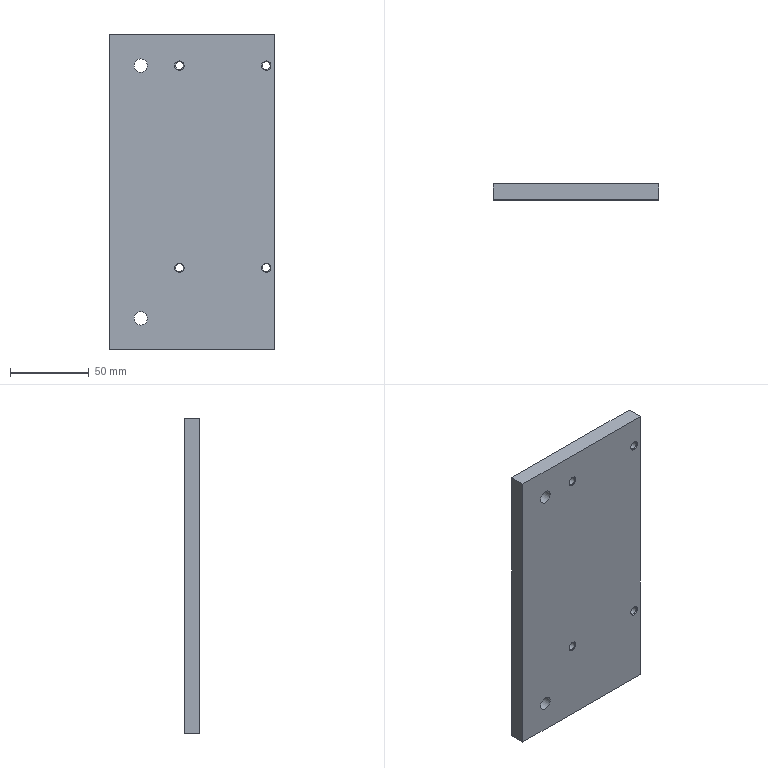Part | STEP file | Button box plate | 1 solid | 20 faces | box 105 x 10 x 200 mm | volume 208063 mm3 | cone 8 | cylinder 6 | plane 6 | commonest cylinder face diameters 5 x4 8.5 x2
STEP:
#1=CARTESIAN_POINT('',(0.,0.,0.));
#2=DIRECTION('',(0.,0.,1.));
#3=DIRECTION('',(1.,0.,0.));
#4=AXIS2_PLACEMENT_3D('',#1,#2,#3);
#5=CARTESIAN_POINT('',(-810.5,-295.,282.25));
#6=VERTEX_POINT('',#5);
#7=CARTESIAN_POINT('',(-810.5,-295.,278.));
#8=DIRECTION('',(0.,-1.,0.));
#9=DIRECTION('',(0.,0.,1.));
#10=AXIS2_PLACEMENT_3D('',#7,#8,#9);
#11=CIRCLE('',#10,4.25);
#12=CARTESIAN_POINT('',(-810.5,-328.,278.));
#13=DIRECTION('',(0.,1.,0.));
#14=DIRECTION('',(0.,0.,1.));
#15=AXIS2_PLACEMENT_3D('',#12,#13,#14);
#16=CYLINDRICAL_SURFACE('',#15,4.25);
#17=CARTESIAN_POINT('',(6.283,33.));
#18=DIRECTION('',(-1.,0.));
#19=VECTOR('',#18,1.);
#20=LINE('',#17,#19);
#21=(GEOMETRIC_REPRESENTATION_CONTEXT(2)PARAMETRIC_REPRESENTATION_CONTEXT()REPRESENTATION_CONTEXT('',''));
#22=DEFINITIONAL_REPRESENTATION('',(#20),#21);
#23=PCURVE('',#16,#22);
#24=CARTESIAN_POINT('',(-783.5,-295.,146.));
#25=DIRECTION('',(0.,1.,0.));
#26=DIRECTION('',(0.,0.,-1.));
#27=AXIS2_PLACEMENT_3D('',#24,#25,#26);
#28=PLANE('',#27);
#29=CARTESIAN_POINT('',(-136.25,27.));
#30=CARTESIAN_POINT('',(-136.25,34.361));
#31=CARTESIAN_POINT('',(-129.875,30.681));
#32=CARTESIAN_POINT('',(-123.5,27.));
#33=CARTESIAN_POINT('',(-129.875,23.319));
#34=CARTESIAN_POINT('',(-136.25,19.639));
#35=CARTESIAN_POINT('',(-136.25,27.));
#36=(BOUNDED_CURVE()B_SPLINE_CURVE(2,(#29,#30,#31,#32,#33,#34,#35),.UNSPECIFIED.,.T.,.F.)B_SPLINE_CURVE_WITH_KNOTS((1,2,2,2,2,1),(-2.094,0.,2.094,4.189,6.283,8.378),.UNSPECIFIED.)CURVE()GEOMETRIC_REPRESENTATION_ITEM()RATIONAL_B_SPLINE_CURVE((1.,0.5,1.,0.5,1.,0.5,1.))REPRESENTATION_ITEM(''));
#37=(GEOMETRIC_REPRESENTATION_CONTEXT(2)PARAMETRIC_REPRESENTATION_CONTEXT()REPRESENTATION_CONTEXT('',''));
#38=DEFINITIONAL_REPRESENTATION('',(#36),#37);
#39=PCURVE('',#28,#38);
#40=SURFACE_CURVE('',#11,(#23,#39),.PCURVE_S1.);
#41=EDGE_CURVE('',#6,#6,#40,.T.);
#42=ORIENTED_EDGE('',*,*,#41,.T.);
#43=CARTESIAN_POINT('',(-810.5,-305.,282.25));
#44=VERTEX_POINT('',#43);
#45=CARTESIAN_POINT('',(-810.5,-305.,282.25));
#46=CARTESIAN_POINT('',(-810.5,-295.,282.25));
#47=B_SPLINE_CURVE_WITH_KNOTS('',1,(#45,#46),.UNSPECIFIED.,.F.,.F.,(2,2),(23.,33.),.PIECEWISE_BEZIER_KNOTS.);
#48=CARTESIAN_POINT('',(0.,0.));
#49=DIRECTION('',(0.,1.));
#50=VECTOR('',#49,1.);
#51=LINE('',#48,#50);
#52=(GEOMETRIC_REPRESENTATION_CONTEXT(2)PARAMETRIC_REPRESENTATION_CONTEXT()REPRESENTATION_CONTEXT('',''));
#53=DEFINITIONAL_REPRESENTATION('',(#51),#52);
#54=PCURVE('',#16,#53);
#55=CARTESIAN_POINT('',(6.283,0.));
#56=DIRECTION('',(0.,1.));
#57=VECTOR('',#56,1.);
#58=LINE('',#55,#57);
#59=(GEOMETRIC_REPRESENTATION_CONTEXT(2)PARAMETRIC_REPRESENTATION_CONTEXT()REPRESENTATION_CONTEXT('',''));
#60=DEFINITIONAL_REPRESENTATION('',(#58),#59);
#61=PCURVE('',#16,#60);
#62=SEAM_CURVE('',#47,(#54,#61),.PCURVE_S1.);
#63=EDGE_CURVE('',#44,#6,#62,.T.);
#64=ORIENTED_EDGE('',*,*,#63,.F.);
#65=CARTESIAN_POINT('',(-810.5,-305.,278.));
#66=DIRECTION('',(0.,1.,0.));
#67=DIRECTION('',(0.,0.,1.));
#68=AXIS2_PLACEMENT_3D('',#65,#66,#67);
#69=CIRCLE('',#68,4.25);
#70=CARTESIAN_POINT('',(0.,23.));
#71=DIRECTION('',(1.,0.));
#72=VECTOR('',#71,1.);
#73=LINE('',#70,#72);
#74=(GEOMETRIC_REPRESENTATION_CONTEXT(2)PARAMETRIC_REPRESENTATION_CONTEXT()REPRESENTATION_CONTEXT('',''));
#75=DEFINITIONAL_REPRESENTATION('',(#73),#74);
#76=PCURVE('',#16,#75);
#77=CARTESIAN_POINT('',(-783.5,-305.,146.));
#78=DIRECTION('',(0.,1.,0.));
#79=DIRECTION('',(0.,0.,-1.));
#80=AXIS2_PLACEMENT_3D('',#77,#78,#79);
#81=PLANE('',#80);
#82=CARTESIAN_POINT('',(-132.,27.));
#83=DIRECTION('',(-1.,0.));
#84=AXIS2_PLACEMENT_2D('',#82,#83);
#85=CIRCLE('',#84,4.25);
#86=(GEOMETRIC_REPRESENTATION_CONTEXT(2)PARAMETRIC_REPRESENTATION_CONTEXT()REPRESENTATION_CONTEXT('',''));
#87=DEFINITIONAL_REPRESENTATION('',(#85),#86);
#88=PCURVE('',#81,#87);
#89=SURFACE_CURVE('',#69,(#76,#88),.PCURVE_S1.);
#90=EDGE_CURVE('',#44,#44,#89,.T.);
#91=ORIENTED_EDGE('',*,*,#90,.T.);
#92=ORIENTED_EDGE('',*,*,#63,.T.);
#93=EDGE_LOOP('',(#42,#64,#91,#92));
#94=FACE_BOUND('',#93,.F.);
#95=ADVANCED_FACE('',(#94),#16,.F.);
#96=CARTESIAN_POINT('',(-830.5,-305.,298.));
#97=VERTEX_POINT('',#96);
#98=CARTESIAN_POINT('',(-725.5,-305.,298.));
#99=VERTEX_POINT('',#98);
#100=CARTESIAN_POINT('',(-1441.,-305.,298.));
#101=DIRECTION('',(1.,0.,0.));
#102=VECTOR('',#101,1.);
#103=LINE('',#100,#102);
#104=CARTESIAN_POINT('',(-1441.,-107.5,298.));
#105=DIRECTION('',(0.,0.,-1.));
#106=DIRECTION('',(-1.,0.,0.));
#107=AXIS2_PLACEMENT_3D('',#104,#105,#106);
#108=PLANE('',#107);
#109=CARTESIAN_POINT('',(0.,-197.5));
#110=DIRECTION('',(-1.,0.));
#111=VECTOR('',#110,1.);
#112=LINE('',#109,#111);
#113=(GEOMETRIC_REPRESENTATION_CONTEXT(2)PARAMETRIC_REPRESENTATION_CONTEXT()REPRESENTATION_CONTEXT('',''));
#114=DEFINITIONAL_REPRESENTATION('',(#112),#113);
#115=PCURVE('',#108,#114);
#116=CARTESIAN_POINT('',(-152.,657.5));
#117=DIRECTION('',(0.,-1.));
#118=VECTOR('',#117,1.);
#119=LINE('',#116,#118);
#120=(GEOMETRIC_REPRESENTATION_CONTEXT(2)PARAMETRIC_REPRESENTATION_CONTEXT()REPRESENTATION_CONTEXT('',''));
#121=DEFINITIONAL_REPRESENTATION('',(#119),#120);
#122=PCURVE('',#81,#121);
#123=SURFACE_CURVE('',#103,(#115,#122),.PCURVE_S1.);
#124=EDGE_CURVE('',#97,#99,#123,.T.);
#125=ORIENTED_EDGE('',*,*,#124,.T.);
#126=CARTESIAN_POINT('',(-725.5,-295.,298.));
#127=VERTEX_POINT('',#126);
#128=CARTESIAN_POINT('',(-725.5,-107.5,298.));
#129=DIRECTION('',(0.,1.,0.));
#130=VECTOR('',#129,1.);
#131=LINE('',#128,#130);
#132=CARTESIAN_POINT('',(-715.5,0.));
#133=DIRECTION('',(0.,1.));
#134=VECTOR('',#133,1.);
#135=LINE('',#132,#134);
#136=(GEOMETRIC_REPRESENTATION_CONTEXT(2)PARAMETRIC_REPRESENTATION_CONTEXT()REPRESENTATION_CONTEXT('',''));
#137=DEFINITIONAL_REPRESENTATION('',(#135),#136);
#138=PCURVE('',#108,#137);
#139=CARTESIAN_POINT('',(-725.5,-295.,146.));
#140=DIRECTION('',(-1.,0.,0.));
#141=DIRECTION('',(0.,1.,0.));
#142=AXIS2_PLACEMENT_3D('',#139,#140,#141);
#143=PLANE('',#142);
#144=CARTESIAN_POINT('',(187.5,-152.));
#145=DIRECTION('',(1.,0.));
#146=VECTOR('',#145,1.);
#147=LINE('',#144,#146);
#148=(GEOMETRIC_REPRESENTATION_CONTEXT(2)PARAMETRIC_REPRESENTATION_CONTEXT()REPRESENTATION_CONTEXT('',''));
#149=DEFINITIONAL_REPRESENTATION('',(#147),#148);
#150=PCURVE('',#143,#149);
#151=SURFACE_CURVE('',#131,(#138,#150),.PCURVE_S1.);
#152=EDGE_CURVE('',#99,#127,#151,.T.);
#153=ORIENTED_EDGE('',*,*,#152,.T.);
#154=CARTESIAN_POINT('',(-830.5,-295.,298.));
#155=VERTEX_POINT('',#154);
#156=CARTESIAN_POINT('',(-1441.,-295.,298.));
#157=DIRECTION('',(1.,0.,0.));
#158=VECTOR('',#157,1.);
#159=LINE('',#156,#158);
#160=CARTESIAN_POINT('',(0.,-187.5));
#161=DIRECTION('',(-1.,0.));
#162=VECTOR('',#161,1.);
#163=LINE('',#160,#162);
#164=(GEOMETRIC_REPRESENTATION_CONTEXT(2)PARAMETRIC_REPRESENTATION_CONTEXT()REPRESENTATION_CONTEXT('',''));
#165=DEFINITIONAL_REPRESENTATION('',(#163),#164);
#166=PCURVE('',#108,#165);
#167=CARTESIAN_POINT('',(-152.,657.5));
#168=DIRECTION('',(0.,-1.));
#169=VECTOR('',#168,1.);
#170=LINE('',#167,#169);
#171=(GEOMETRIC_REPRESENTATION_CONTEXT(2)PARAMETRIC_REPRESENTATION_CONTEXT()REPRESENTATION_CONTEXT('',''));
#172=DEFINITIONAL_REPRESENTATION('',(#170),#171);
#173=PCURVE('',#28,#172);
#174=SURFACE_CURVE('',#159,(#166,#173),.PCURVE_S1.);
#175=EDGE_CURVE('',#155,#127,#174,.T.);
#176=ORIENTED_EDGE('',*,*,#175,.F.);
#177=CARTESIAN_POINT('',(-830.5,-295.,298.));
#178=DIRECTION('',(0.,1.,0.));
#179=VECTOR('',#178,1.);
#180=LINE('',#177,#179);
#181=CARTESIAN_POINT('',(-610.5,-187.5));
#182=DIRECTION('',(0.,1.));
#183=VECTOR('',#182,1.);
#184=LINE('',#181,#183);
#185=(GEOMETRIC_REPRESENTATION_CONTEXT(2)PARAMETRIC_REPRESENTATION_CONTEXT()REPRESENTATION_CONTEXT('',''));
#186=DEFINITIONAL_REPRESENTATION('',(#184),#185);
#187=PCURVE('',#108,#186);
#188=CARTESIAN_POINT('',(-830.5,-295.,294.));
#189=DIRECTION('',(1.,0.,0.));
#190=DIRECTION('',(0.,-1.,0.));
#191=AXIS2_PLACEMENT_3D('',#188,#189,#190);
#192=PLANE('',#191);
#193=CARTESIAN_POINT('',(0.,-4.));
#194=DIRECTION('',(-1.,0.));
#195=VECTOR('',#194,1.);
#196=LINE('',#193,#195);
#197=(GEOMETRIC_REPRESENTATION_CONTEXT(2)PARAMETRIC_REPRESENTATION_CONTEXT()REPRESENTATION_CONTEXT('',''));
#198=DEFINITIONAL_REPRESENTATION('',(#196),#197);
#199=PCURVE('',#192,#198);
#200=SURFACE_CURVE('',#180,(#187,#199),.PCURVE_S1.);
#201=EDGE_CURVE('',#97,#155,#200,.T.);
#202=ORIENTED_EDGE('',*,*,#201,.F.);
#203=EDGE_LOOP('',(#125,#153,#176,#202));
#204=FACE_BOUND('',#203,.T.);
#205=ADVANCED_FACE('',(#204),#108,.F.);
#206=CARTESIAN_POINT('',(-725.5,-305.,98.));
#207=VERTEX_POINT('',#206);
#208=CARTESIAN_POINT('',(-725.5,-305.,146.));
#209=DIRECTION('',(0.,0.,-1.));
#210=VECTOR('',#209,1.);
#211=LINE('',#208,#210);
#212=CARTESIAN_POINT('',(-10.,0.));
#213=DIRECTION('',(0.,1.));
#214=VECTOR('',#213,1.);
#215=LINE('',#212,#214);
#216=(GEOMETRIC_REPRESENTATION_CONTEXT(2)PARAMETRIC_REPRESENTATION_CONTEXT()REPRESENTATION_CONTEXT('',''));
#217=DEFINITIONAL_REPRESENTATION('',(#215),#216);
#218=PCURVE('',#143,#217);
#219=CARTESIAN_POINT('',(0.,-58.));
#220=DIRECTION('',(1.,0.));
#221=VECTOR('',#220,1.);
#222=LINE('',#219,#221);
#223=(GEOMETRIC_REPRESENTATION_CONTEXT(2)PARAMETRIC_REPRESENTATION_CONTEXT()REPRESENTATION_CONTEXT('',''));
#224=DEFINITIONAL_REPRESENTATION('',(#222),#223);
#225=PCURVE('',#81,#224);
#226=SURFACE_CURVE('',#211,(#218,#225),.PCURVE_S1.);
#227=EDGE_CURVE('',#99,#207,#226,.T.);
#228=ORIENTED_EDGE('',*,*,#227,.T.);
#229=CARTESIAN_POINT('',(-725.5,-295.,98.));
#230=VERTEX_POINT('',#229);
#231=CARTESIAN_POINT('',(-725.5,-295.,98.));
#232=DIRECTION('',(0.,1.,0.));
#233=VECTOR('',#232,1.);
#234=LINE('',#231,#233);
#235=CARTESIAN_POINT('',(0.,48.));
#236=DIRECTION('',(1.,0.));
#237=VECTOR('',#236,1.);
#238=LINE('',#235,#237);
#239=(GEOMETRIC_REPRESENTATION_CONTEXT(2)PARAMETRIC_REPRESENTATION_CONTEXT()REPRESENTATION_CONTEXT('',''));
#240=DEFINITIONAL_REPRESENTATION('',(#238),#239);
#241=PCURVE('',#143,#240);
#242=CARTESIAN_POINT('',(-798.5,-375.,98.));
#243=DIRECTION('',(0.,0.,1.));
#244=DIRECTION('',(0.,1.,0.));
#245=AXIS2_PLACEMENT_3D('',#242,#243,#244);
#246=PLANE('',#245);
#247=CARTESIAN_POINT('',(80.,-73.));
#248=DIRECTION('',(1.,0.));
#249=VECTOR('',#248,1.);
#250=LINE('',#247,#249);
#251=(GEOMETRIC_REPRESENTATION_CONTEXT(2)PARAMETRIC_REPRESENTATION_CONTEXT()REPRESENTATION_CONTEXT('',''));
#252=DEFINITIONAL_REPRESENTATION('',(#250),#251);
#253=PCURVE('',#246,#252);
#254=SURFACE_CURVE('',#234,(#241,#253),.PCURVE_S1.);
#255=EDGE_CURVE('',#207,#230,#254,.T.);
#256=ORIENTED_EDGE('',*,*,#255,.T.);
#257=CARTESIAN_POINT('',(-725.5,-295.,146.));
#258=DIRECTION('',(0.,0.,-1.));
#259=VECTOR('',#258,1.);
#260=LINE('',#257,#259);
#261=CARTESIAN_POINT('',(0.,0.));
#262=DIRECTION('',(0.,1.));
#263=VECTOR('',#262,1.);
#264=LINE('',#261,#263);
#265=(GEOMETRIC_REPRESENTATION_CONTEXT(2)PARAMETRIC_REPRESENTATION_CONTEXT()REPRESENTATION_CONTEXT('',''));
#266=DEFINITIONAL_REPRESENTATION('',(#264),#265);
#267=PCURVE('',#143,#266);
#268=CARTESIAN_POINT('',(0.,-58.));
#269=DIRECTION('',(1.,0.));
#270=VECTOR('',#269,1.);
#271=LINE('',#268,#270);
#272=(GEOMETRIC_REPRESENTATION_CONTEXT(2)PARAMETRIC_REPRESENTATION_CONTEXT()REPRESENTATION_CONTEXT('',''));
#273=DEFINITIONAL_REPRESENTATION('',(#271),#272);
#274=PCURVE('',#28,#273);
#275=SURFACE_CURVE('',#260,(#267,#274),.PCURVE_S1.);
#276=EDGE_CURVE('',#127,#230,#275,.T.);
#277=ORIENTED_EDGE('',*,*,#276,.F.);
#278=ORIENTED_EDGE('',*,*,#152,.F.);
#279=EDGE_LOOP('',(#228,#256,#277,#278));
#280=FACE_BOUND('',#279,.T.);
#281=ADVANCED_FACE('',(#280),#143,.F.);
#282=CARTESIAN_POINT('',(-830.5,-305.,98.));
#283=VERTEX_POINT('',#282);
#284=CARTESIAN_POINT('',(-798.5,-305.,98.));
#285=DIRECTION('',(-1.,0.,0.));
#286=VECTOR('',#285,1.);
#287=LINE('',#284,#286);
#288=CARTESIAN_POINT('',(70.,0.));
#289=DIRECTION('',(0.,1.));
#290=VECTOR('',#289,1.);
#291=LINE('',#288,#290);
#292=(GEOMETRIC_REPRESENTATION_CONTEXT(2)PARAMETRIC_REPRESENTATION_CONTEXT()REPRESENTATION_CONTEXT('',''));
#293=DEFINITIONAL_REPRESENTATION('',(#291),#292);
#294=PCURVE('',#246,#293);
#295=CARTESIAN_POINT('',(48.,15.));
#296=DIRECTION('',(0.,1.));
#297=VECTOR('',#296,1.);
#298=LINE('',#295,#297);
#299=(GEOMETRIC_REPRESENTATION_CONTEXT(2)PARAMETRIC_REPRESENTATION_CONTEXT()REPRESENTATION_CONTEXT('',''));
#300=DEFINITIONAL_REPRESENTATION('',(#298),#299);
#301=PCURVE('',#81,#300);
#302=SURFACE_CURVE('',#287,(#294,#301),.PCURVE_S1.);
#303=EDGE_CURVE('',#207,#283,#302,.T.);
#304=ORIENTED_EDGE('',*,*,#303,.T.);
#305=CARTESIAN_POINT('',(-830.5,-295.,98.));
#306=VERTEX_POINT('',#305);
#307=CARTESIAN_POINT('',(-830.5,-375.,98.));
#308=DIRECTION('',(0.,1.,0.));
#309=VECTOR('',#308,1.);
#310=LINE('',#307,#309);
#311=CARTESIAN_POINT('',(0.,32.));
#312=DIRECTION('',(1.,0.));
#313=VECTOR('',#312,1.);
#314=LINE('',#311,#313);
#315=(GEOMETRIC_REPRESENTATION_CONTEXT(2)PARAMETRIC_REPRESENTATION_CONTEXT()REPRESENTATION_CONTEXT('',''));
#316=DEFINITIONAL_REPRESENTATION('',(#314),#315);
#317=PCURVE('',#246,#316);
#318=CARTESIAN_POINT('',(80.,196.));
#319=DIRECTION('',(-1.,0.));
#320=VECTOR('',#319,1.);
#321=LINE('',#318,#320);
#322=(GEOMETRIC_REPRESENTATION_CONTEXT(2)PARAMETRIC_REPRESENTATION_CONTEXT()REPRESENTATION_CONTEXT('',''));
#323=DEFINITIONAL_REPRESENTATION('',(#321),#322);
#324=PCURVE('',#192,#323);
#325=SURFACE_CURVE('',#310,(#317,#324),.PCURVE_S1.);
#326=EDGE_CURVE('',#283,#306,#325,.T.);
#327=ORIENTED_EDGE('',*,*,#326,.T.);
#328=CARTESIAN_POINT('',(-798.5,-295.,98.));
#329=DIRECTION('',(-1.,0.,0.));
#330=VECTOR('',#329,1.);
#331=LINE('',#328,#330);
#332=CARTESIAN_POINT('',(80.,0.));
#333=DIRECTION('',(0.,1.));
#334=VECTOR('',#333,1.);
#335=LINE('',#332,#334);
#336=(GEOMETRIC_REPRESENTATION_CONTEXT(2)PARAMETRIC_REPRESENTATION_CONTEXT()REPRESENTATION_CONTEXT('',''));
#337=DEFINITIONAL_REPRESENTATION('',(#335),#336);
#338=PCURVE('',#246,#337);
#339=CARTESIAN_POINT('',(48.,15.));
#340=DIRECTION('',(0.,1.));
#341=VECTOR('',#340,1.);
#342=LINE('',#339,#341);
#343=(GEOMETRIC_REPRESENTATION_CONTEXT(2)PARAMETRIC_REPRESENTATION_CONTEXT()REPRESENTATION_CONTEXT('',''));
#344=DEFINITIONAL_REPRESENTATION('',(#342),#343);
#345=PCURVE('',#28,#344);
#346=SURFACE_CURVE('',#331,(#338,#345),.PCURVE_S1.);
#347=EDGE_CURVE('',#230,#306,#346,.T.);
#348=ORIENTED_EDGE('',*,*,#347,.F.);
#349=ORIENTED_EDGE('',*,*,#255,.F.);
#350=EDGE_LOOP('',(#304,#327,#348,#349));
#351=FACE_BOUND('',#350,.T.);
#352=ADVANCED_FACE('',(#351),#246,.F.);
#353=CARTESIAN_POINT('',(-830.5,-305.,294.));
#354=DIRECTION('',(0.,0.,1.));
#355=VECTOR('',#354,1.);
#356=LINE('',#353,#355);
#357=CARTESIAN_POINT('',(10.,0.));
#358=DIRECTION('',(0.,-1.));
#359=VECTOR('',#358,1.);
#360=LINE('',#357,#359);
#361=(GEOMETRIC_REPRESENTATION_CONTEXT(2)PARAMETRIC_REPRESENTATION_CONTEXT()REPRESENTATION_CONTEXT('',''));
#362=DEFINITIONAL_REPRESENTATION('',(#360),#361);
#363=PCURVE('',#192,#362);
#364=CARTESIAN_POINT('',(-148.,47.));
#365=DIRECTION('',(-1.,0.));
#366=VECTOR('',#365,1.);
#367=LINE('',#364,#366);
#368=(GEOMETRIC_REPRESENTATION_CONTEXT(2)PARAMETRIC_REPRESENTATION_CONTEXT()REPRESENTATION_CONTEXT('',''));
#369=DEFINITIONAL_REPRESENTATION('',(#367),#368);
#370=PCURVE('',#81,#369);
#371=SURFACE_CURVE('',#356,(#363,#370),.PCURVE_S1.);
#372=EDGE_CURVE('',#283,#97,#371,.T.);
#373=ORIENTED_EDGE('',*,*,#372,.T.);
#374=ORIENTED_EDGE('',*,*,#201,.T.);
#375=CARTESIAN_POINT('',(-830.5,-295.,294.));
#376=DIRECTION('',(0.,0.,1.));
#377=VECTOR('',#376,1.);
#378=LINE('',#375,#377);
#379=CARTESIAN_POINT('',(0.,0.));
#380=DIRECTION('',(0.,-1.));
#381=VECTOR('',#380,1.);
#382=LINE('',#379,#381);
#383=(GEOMETRIC_REPRESENTATION_CONTEXT(2)PARAMETRIC_REPRESENTATION_CONTEXT()REPRESENTATION_CONTEXT('',''));
#384=DEFINITIONAL_REPRESENTATION('',(#382),#383);
#385=PCURVE('',#192,#384);
#386=CARTESIAN_POINT('',(-148.,47.));
#387=DIRECTION('',(-1.,0.));
#388=VECTOR('',#387,1.);
#389=LINE('',#386,#388);
#390=(GEOMETRIC_REPRESENTATION_CONTEXT(2)PARAMETRIC_REPRESENTATION_CONTEXT()REPRESENTATION_CONTEXT('',''));
#391=DEFINITIONAL_REPRESENTATION('',(#389),#390);
#392=PCURVE('',#28,#391);
#393=SURFACE_CURVE('',#378,(#385,#392),.PCURVE_S1.);
#394=EDGE_CURVE('',#306,#155,#393,.T.);
#395=ORIENTED_EDGE('',*,*,#394,.F.);
#396=ORIENTED_EDGE('',*,*,#326,.F.);
#397=EDGE_LOOP('',(#373,#374,#395,#396));
#398=FACE_BOUND('',#397,.T.);
#399=ADVANCED_FACE('',(#398),#192,.F.);
#400=CARTESIAN_POINT('',(-786.,-305.,281.));
#401=VERTEX_POINT('',#400);
#402=CARTESIAN_POINT('',(-786.,-305.,278.));
#403=DIRECTION('',(0.,1.,0.));
#404=DIRECTION('',(0.,0.,1.));
#405=AXIS2_PLACEMENT_3D('',#402,#403,#404);
#406=CIRCLE('',#405,3.);
#407=CARTESIAN_POINT('',(-132.,2.5));
#408=DIRECTION('',(-1.,0.));
#409=AXIS2_PLACEMENT_2D('',#407,#408);
#410=CIRCLE('',#409,3.);
#411=(GEOMETRIC_REPRESENTATION_CONTEXT(2)PARAMETRIC_REPRESENTATION_CONTEXT()REPRESENTATION_CONTEXT('',''));
#412=DEFINITIONAL_REPRESENTATION('',(#410),#411);
#413=PCURVE('',#81,#412);
#414=CARTESIAN_POINT('',(-786.,-304.5,278.));
#415=DIRECTION('',(0.,-1.,0.));
#416=DIRECTION('',(0.,0.,-1.));
#417=AXIS2_PLACEMENT_3D('',#414,#415,#416);
#418=CONICAL_SURFACE('',#417,2.5,0.7854);
#419=CARTESIAN_POINT('',(9.425,0.5));
#420=DIRECTION('',(-1.,0.));
#421=VECTOR('',#420,1.);
#422=LINE('',#419,#421);
#423=(GEOMETRIC_REPRESENTATION_CONTEXT(2)PARAMETRIC_REPRESENTATION_CONTEXT()REPRESENTATION_CONTEXT('',''));
#424=DEFINITIONAL_REPRESENTATION('',(#422),#423);
#425=PCURVE('',#418,#424);
#426=SURFACE_CURVE('',#406,(#413,#425),.PCURVE_S1.);
#427=EDGE_CURVE('',#401,#401,#426,.T.);
#428=ORIENTED_EDGE('',*,*,#427,.T.);
#429=EDGE_LOOP('',(#428));
#430=FACE_BOUND('',#429,.T.);
#431=CARTESIAN_POINT('',(-731.,-305.,281.));
#432=VERTEX_POINT('',#431);
#433=CARTESIAN_POINT('',(-731.,-305.,278.));
#434=DIRECTION('',(0.,1.,0.));
#435=DIRECTION('',(0.,0.,1.));
#436=AXIS2_PLACEMENT_3D('',#433,#434,#435);
#437=CIRCLE('',#436,3.);
#438=CARTESIAN_POINT('',(-132.,-52.5));
#439=DIRECTION('',(-1.,0.));
#440=AXIS2_PLACEMENT_2D('',#438,#439);
#441=CIRCLE('',#440,3.);
#442=(GEOMETRIC_REPRESENTATION_CONTEXT(2)PARAMETRIC_REPRESENTATION_CONTEXT()REPRESENTATION_CONTEXT('',''));
#443=DEFINITIONAL_REPRESENTATION('',(#441),#442);
#444=PCURVE('',#81,#443);
#445=CARTESIAN_POINT('',(-731.,-304.5,278.));
#446=DIRECTION('',(0.,-1.,0.));
#447=DIRECTION('',(0.,0.,-1.));
#448=AXIS2_PLACEMENT_3D('',#445,#446,#447);
#449=CONICAL_SURFACE('',#448,2.5,0.7854);
#450=CARTESIAN_POINT('',(9.425,0.5));
#451=DIRECTION('',(-1.,0.));
#452=VECTOR('',#451,1.);
#453=LINE('',#450,#452);
#454=(GEOMETRIC_REPRESENTATION_CONTEXT(2)PARAMETRIC_REPRESENTATION_CONTEXT()REPRESENTATION_CONTEXT('',''));
#455=DEFINITIONAL_REPRESENTATION('',(#453),#454);
#456=PCURVE('',#449,#455);
#457=SURFACE_CURVE('',#437,(#444,#456),.PCURVE_S1.);
#458=EDGE_CURVE('',#432,#432,#457,.T.);
#459=ORIENTED_EDGE('',*,*,#458,.T.);
#460=EDGE_LOOP('',(#459));
#461=FACE_BOUND('',#460,.T.);
#462=CARTESIAN_POINT('',(-731.,-305.,153.));
#463=VERTEX_POINT('',#462);
#464=CARTESIAN_POINT('',(-731.,-305.,150.));
#465=DIRECTION('',(0.,1.,0.));
#466=DIRECTION('',(0.,0.,1.));
#467=AXIS2_PLACEMENT_3D('',#464,#465,#466);
#468=CIRCLE('',#467,3.);
#469=CARTESIAN_POINT('',(-4.,-52.5));
#470=DIRECTION('',(-1.,0.));
#471=AXIS2_PLACEMENT_2D('',#469,#470);
#472=CIRCLE('',#471,3.);
#473=(GEOMETRIC_REPRESENTATION_CONTEXT(2)PARAMETRIC_REPRESENTATION_CONTEXT()REPRESENTATION_CONTEXT('',''));
#474=DEFINITIONAL_REPRESENTATION('',(#472),#473);
#475=PCURVE('',#81,#474);
#476=CARTESIAN_POINT('',(-731.,-304.5,150.));
#477=DIRECTION('',(0.,-1.,0.));
#478=DIRECTION('',(0.,0.,-1.));
#479=AXIS2_PLACEMENT_3D('',#476,#477,#478);
#480=CONICAL_SURFACE('',#479,2.5,0.7854);
#481=CARTESIAN_POINT('',(9.425,0.5));
#482=DIRECTION('',(-1.,0.));
#483=VECTOR('',#482,1.);
#484=LINE('',#481,#483);
#485=(GEOMETRIC_REPRESENTATION_CONTEXT(2)PARAMETRIC_REPRESENTATION_CONTEXT()REPRESENTATION_CONTEXT('',''));
#486=DEFINITIONAL_REPRESENTATION('',(#484),#485);
#487=PCURVE('',#480,#486);
#488=SURFACE_CURVE('',#468,(#475,#487),.PCURVE_S1.);
#489=EDGE_CURVE('',#463,#463,#488,.T.);
#490=ORIENTED_EDGE('',*,*,#489,.T.);
#491=EDGE_LOOP('',(#490));
#492=FACE_BOUND('',#491,.T.);
#493=CARTESIAN_POINT('',(-786.,-305.,153.));
#494=VERTEX_POINT('',#493);
#495=CARTESIAN_POINT('',(-786.,-305.,150.));
#496=DIRECTION('',(0.,1.,0.));
#497=DIRECTION('',(0.,0.,1.));
#498=AXIS2_PLACEMENT_3D('',#495,#496,#497);
#499=CIRCLE('',#498,3.);
#500=CARTESIAN_POINT('',(-4.,2.5));
#501=DIRECTION('',(-1.,0.));
#502=AXIS2_PLACEMENT_2D('',#500,#501);
#503=CIRCLE('',#502,3.);
#504=(GEOMETRIC_REPRESENTATION_CONTEXT(2)PARAMETRIC_REPRESENTATION_CONTEXT()REPRESENTATION_CONTEXT('',''));
#505=DEFINITIONAL_REPRESENTATION('',(#503),#504);
#506=PCURVE('',#81,#505);
#507=CARTESIAN_POINT('',(-786.,-304.5,150.));
#508=DIRECTION('',(0.,-1.,0.));
#509=DIRECTION('',(0.,0.,-1.));
#510=AXIS2_PLACEMENT_3D('',#507,#508,#509);
#511=CONICAL_SURFACE('',#510,2.5,0.7854);
#512=CARTESIAN_POINT('',(9.425,0.5));
#513=DIRECTION('',(-1.,0.));
#514=VECTOR('',#513,1.);
#515=LINE('',#512,#514);
#516=(GEOMETRIC_REPRESENTATION_CONTEXT(2)PARAMETRIC_REPRESENTATION_CONTEXT()REPRESENTATION_CONTEXT('',''));
#517=DEFINITIONAL_REPRESENTATION('',(#515),#516);
#518=PCURVE('',#511,#517);
#519=SURFACE_CURVE('',#499,(#506,#518),.PCURVE_S1.);
#520=EDGE_CURVE('',#494,#494,#519,.T.);
#521=ORIENTED_EDGE('',*,*,#520,.T.);
#522=EDGE_LOOP('',(#521));
#523=FACE_BOUND('',#522,.T.);
#524=CARTESIAN_POINT('',(-810.5,-305.,122.25));
#525=VERTEX_POINT('',#524);
#526=CARTESIAN_POINT('',(-810.5,-305.,118.));
#527=DIRECTION('',(0.,1.,0.));
#528=DIRECTION('',(0.,0.,1.));
#529=AXIS2_PLACEMENT_3D('',#526,#527,#528);
#530=CIRCLE('',#529,4.25);
#531=CARTESIAN_POINT('',(28.,27.));
#532=DIRECTION('',(-1.,0.));
#533=AXIS2_PLACEMENT_2D('',#531,#532);
#534=CIRCLE('',#533,4.25);
#535=(GEOMETRIC_REPRESENTATION_CONTEXT(2)PARAMETRIC_REPRESENTATION_CONTEXT()REPRESENTATION_CONTEXT('',''));
#536=DEFINITIONAL_REPRESENTATION('',(#534),#535);
#537=PCURVE('',#81,#536);
#538=CARTESIAN_POINT('',(-810.5,-328.,118.));
#539=DIRECTION('',(0.,1.,0.));
#540=DIRECTION('',(0.,0.,1.));
#541=AXIS2_PLACEMENT_3D('',#538,#539,#540);
#542=CYLINDRICAL_SURFACE('',#541,4.25);
#543=CARTESIAN_POINT('',(0.,23.));
#544=DIRECTION('',(1.,0.));
#545=VECTOR('',#544,1.);
#546=LINE('',#543,#545);
#547=(GEOMETRIC_REPRESENTATION_CONTEXT(2)PARAMETRIC_REPRESENTATION_CONTEXT()REPRESENTATION_CONTEXT('',''));
#548=DEFINITIONAL_REPRESENTATION('',(#546),#547);
#549=PCURVE('',#542,#548);
#550=SURFACE_CURVE('',#530,(#537,#549),.PCURVE_S1.);
#551=EDGE_CURVE('',#525,#525,#550,.T.);
#552=ORIENTED_EDGE('',*,*,#551,.T.);
#553=EDGE_LOOP('',(#552));
#554=FACE_BOUND('',#553,.T.);
#555=ORIENTED_EDGE('',*,*,#90,.T.);
#556=EDGE_LOOP('',(#555));
#557=FACE_BOUND('',#556,.T.);
#558=ORIENTED_EDGE('',*,*,#372,.F.);
#559=ORIENTED_EDGE('',*,*,#303,.F.);
#560=ORIENTED_EDGE('',*,*,#227,.F.);
#561=ORIENTED_EDGE('',*,*,#124,.F.);
#562=EDGE_LOOP('',(#558,#559,#560,#561));
#563=FACE_BOUND('',#562,.T.);
#564=ADVANCED_FACE('',(#430,#461,#492,#523,#554,#557,#563),#81,.F.);
#565=CARTESIAN_POINT('',(-786.,-295.,281.));
#566=VERTEX_POINT('',#565);
#567=CARTESIAN_POINT('',(-786.,-295.,278.));
#568=DIRECTION('',(0.,-1.,0.));
#569=DIRECTION('',(0.,0.,1.));
#570=AXIS2_PLACEMENT_3D('',#567,#568,#569);
#571=CIRCLE('',#570,3.);
#572=CARTESIAN_POINT('',(-135.,2.5));
#573=CARTESIAN_POINT('',(-135.,7.696));
#574=CARTESIAN_POINT('',(-130.5,5.098));
#575=CARTESIAN_POINT('',(-126.,2.5));
#576=CARTESIAN_POINT('',(-130.5,-0.09808));
#577=CARTESIAN_POINT('',(-135.,-2.696));
#578=CARTESIAN_POINT('',(-135.,2.5));
#579=(BOUNDED_CURVE()B_SPLINE_CURVE(2,(#572,#573,#574,#575,#576,#577,#578),.UNSPECIFIED.,.T.,.F.)B_SPLINE_CURVE_WITH_KNOTS((1,2,2,2,2,1),(-2.094,0.,2.094,4.189,6.283,8.378),.UNSPECIFIED.)CURVE()GEOMETRIC_REPRESENTATION_ITEM()RATIONAL_B_SPLINE_CURVE((1.,0.5,1.,0.5,1.,0.5,1.))REPRESENTATION_ITEM(''));
#580=(GEOMETRIC_REPRESENTATION_CONTEXT(2)PARAMETRIC_REPRESENTATION_CONTEXT()REPRESENTATION_CONTEXT('',''));
#581=DEFINITIONAL_REPRESENTATION('',(#579),#580);
#582=PCURVE('',#28,#581);
#583=CARTESIAN_POINT('',(-786.,-295.,278.));
#584=DIRECTION('',(0.,1.,0.));
#585=DIRECTION('',(0.,0.,1.));
#586=AXIS2_PLACEMENT_3D('',#583,#584,#585);
#587=CONICAL_SURFACE('',#586,3.,0.7854);
#588=CARTESIAN_POINT('',(6.283,0.));
#589=DIRECTION('',(-1.,0.));
#590=VECTOR('',#589,1.);
#591=LINE('',#588,#590);
#592=(GEOMETRIC_REPRESENTATION_CONTEXT(2)PARAMETRIC_REPRESENTATION_CONTEXT()REPRESENTATION_CONTEXT('',''));
#593=DEFINITIONAL_REPRESENTATION('',(#591),#592);
#594=PCURVE('',#587,#593);
#595=SURFACE_CURVE('',#571,(#582,#594),.PCURVE_S1.);
#596=EDGE_CURVE('',#566,#566,#595,.T.);
#597=ORIENTED_EDGE('',*,*,#596,.T.);
#598=EDGE_LOOP('',(#597));
#599=FACE_BOUND('',#598,.T.);
#600=CARTESIAN_POINT('',(-731.,-295.,281.));
#601=VERTEX_POINT('',#600);
#602=CARTESIAN_POINT('',(-731.,-295.,278.));
#603=DIRECTION('',(0.,-1.,0.));
#604=DIRECTION('',(0.,0.,1.));
#605=AXIS2_PLACEMENT_3D('',#602,#603,#604);
#606=CIRCLE('',#605,3.);
#607=CARTESIAN_POINT('',(-135.,-52.5));
#608=CARTESIAN_POINT('',(-135.,-47.304));
#609=CARTESIAN_POINT('',(-130.5,-49.902));
#610=CARTESIAN_POINT('',(-126.,-52.5));
#611=CARTESIAN_POINT('',(-130.5,-55.098));
#612=CARTESIAN_POINT('',(-135.,-57.696));
#613=CARTESIAN_POINT('',(-135.,-52.5));
#614=(BOUNDED_CURVE()B_SPLINE_CURVE(2,(#607,#608,#609,#610,#611,#612,#613),.UNSPECIFIED.,.T.,.F.)B_SPLINE_CURVE_WITH_KNOTS((1,2,2,2,2,1),(-2.094,0.,2.094,4.189,6.283,8.378),.UNSPECIFIED.)CURVE()GEOMETRIC_REPRESENTATION_ITEM()RATIONAL_B_SPLINE_CURVE((1.,0.5,1.,0.5,1.,0.5,1.))REPRESENTATION_ITEM(''));
#615=(GEOMETRIC_REPRESENTATION_CONTEXT(2)PARAMETRIC_REPRESENTATION_CONTEXT()REPRESENTATION_CONTEXT('',''));
#616=DEFINITIONAL_REPRESENTATION('',(#614),#615);
#617=PCURVE('',#28,#616);
#618=CARTESIAN_POINT('',(-731.,-295.,278.));
#619=DIRECTION('',(0.,1.,0.));
#620=DIRECTION('',(0.,0.,1.));
#621=AXIS2_PLACEMENT_3D('',#618,#619,#620);
#622=CONICAL_SURFACE('',#621,3.,0.7854);
#623=CARTESIAN_POINT('',(6.283,0.));
#624=DIRECTION('',(-1.,0.));
#625=VECTOR('',#624,1.);
#626=LINE('',#623,#625);
#627=(GEOMETRIC_REPRESENTATION_CONTEXT(2)PARAMETRIC_REPRESENTATION_CONTEXT()REPRESENTATION_CONTEXT('',''));
#628=DEFINITIONAL_REPRESENTATION('',(#626),#627);
#629=PCURVE('',#622,#628);
#630=SURFACE_CURVE('',#606,(#617,#629),.PCURVE_S1.);
#631=EDGE_CURVE('',#601,#601,#630,.T.);
#632=ORIENTED_EDGE('',*,*,#631,.T.);
#633=EDGE_LOOP('',(#632));
#634=FACE_BOUND('',#633,.T.);
#635=CARTESIAN_POINT('',(-731.,-295.,153.));
#636=VERTEX_POINT('',#635);
#637=CARTESIAN_POINT('',(-731.,-295.,150.));
#638=DIRECTION('',(0.,-1.,0.));
#639=DIRECTION('',(0.,0.,1.));
#640=AXIS2_PLACEMENT_3D('',#637,#638,#639);
#641=CIRCLE('',#640,3.);
#642=CARTESIAN_POINT('',(-7.,-52.5));
#643=CARTESIAN_POINT('',(-7.,-47.304));
#644=CARTESIAN_POINT('',(-2.5,-49.902));
#645=CARTESIAN_POINT('',(2.,-52.5));
#646=CARTESIAN_POINT('',(-2.5,-55.098));
#647=CARTESIAN_POINT('',(-7.,-57.696));
#648=CARTESIAN_POINT('',(-7.,-52.5));
#649=(BOUNDED_CURVE()B_SPLINE_CURVE(2,(#642,#643,#644,#645,#646,#647,#648),.UNSPECIFIED.,.T.,.F.)B_SPLINE_CURVE_WITH_KNOTS((1,2,2,2,2,1),(-2.094,0.,2.094,4.189,6.283,8.378),.UNSPECIFIED.)CURVE()GEOMETRIC_REPRESENTATION_ITEM()RATIONAL_B_SPLINE_CURVE((1.,0.5,1.,0.5,1.,0.5,1.))REPRESENTATION_ITEM(''));
#650=(GEOMETRIC_REPRESENTATION_CONTEXT(2)PARAMETRIC_REPRESENTATION_CONTEXT()REPRESENTATION_CONTEXT('',''));
#651=DEFINITIONAL_REPRESENTATION('',(#649),#650);
#652=PCURVE('',#28,#651);
#653=CARTESIAN_POINT('',(-731.,-295.,150.));
#654=DIRECTION('',(0.,1.,0.));
#655=DIRECTION('',(0.,0.,1.));
#656=AXIS2_PLACEMENT_3D('',#653,#654,#655);
#657=CONICAL_SURFACE('',#656,3.,0.7854);
#658=CARTESIAN_POINT('',(6.283,0.));
#659=DIRECTION('',(-1.,0.));
#660=VECTOR('',#659,1.);
#661=LINE('',#658,#660);
#662=(GEOMETRIC_REPRESENTATION_CONTEXT(2)PARAMETRIC_REPRESENTATION_CONTEXT()REPRESENTATION_CONTEXT('',''));
#663=DEFINITIONAL_REPRESENTATION('',(#661),#662);
#664=PCURVE('',#657,#663);
#665=SURFACE_CURVE('',#641,(#652,#664),.PCURVE_S1.);
#666=EDGE_CURVE('',#636,#636,#665,.T.);
#667=ORIENTED_EDGE('',*,*,#666,.T.);
#668=EDGE_LOOP('',(#667));
#669=FACE_BOUND('',#668,.T.);
#670=CARTESIAN_POINT('',(-786.,-295.,153.));
#671=VERTEX_POINT('',#670);
#672=CARTESIAN_POINT('',(-786.,-295.,150.));
#673=DIRECTION('',(0.,-1.,0.));
#674=DIRECTION('',(0.,0.,1.));
#675=AXIS2_PLACEMENT_3D('',#672,#673,#674);
#676=CIRCLE('',#675,3.);
#677=CARTESIAN_POINT('',(-7.,2.5));
#678=CARTESIAN_POINT('',(-7.,7.696));
#679=CARTESIAN_POINT('',(-2.5,5.098));
#680=CARTESIAN_POINT('',(2.,2.5));
#681=CARTESIAN_POINT('',(-2.5,-0.09808));
#682=CARTESIAN_POINT('',(-7.,-2.696));
#683=CARTESIAN_POINT('',(-7.,2.5));
#684=(BOUNDED_CURVE()B_SPLINE_CURVE(2,(#677,#678,#679,#680,#681,#682,#683),.UNSPECIFIED.,.T.,.F.)B_SPLINE_CURVE_WITH_KNOTS((1,2,2,2,2,1),(-2.094,0.,2.094,4.189,6.283,8.378),.UNSPECIFIED.)CURVE()GEOMETRIC_REPRESENTATION_ITEM()RATIONAL_B_SPLINE_CURVE((1.,0.5,1.,0.5,1.,0.5,1.))REPRESENTATION_ITEM(''));
#685=(GEOMETRIC_REPRESENTATION_CONTEXT(2)PARAMETRIC_REPRESENTATION_CONTEXT()REPRESENTATION_CONTEXT('',''));
#686=DEFINITIONAL_REPRESENTATION('',(#684),#685);
#687=PCURVE('',#28,#686);
#688=CARTESIAN_POINT('',(-786.,-295.,150.));
#689=DIRECTION('',(0.,1.,0.));
#690=DIRECTION('',(0.,0.,1.));
#691=AXIS2_PLACEMENT_3D('',#688,#689,#690);
#692=CONICAL_SURFACE('',#691,3.,0.7854);
#693=CARTESIAN_POINT('',(6.283,0.));
#694=DIRECTION('',(-1.,0.));
#695=VECTOR('',#694,1.);
#696=LINE('',#693,#695);
#697=(GEOMETRIC_REPRESENTATION_CONTEXT(2)PARAMETRIC_REPRESENTATION_CONTEXT()REPRESENTATION_CONTEXT('',''));
#698=DEFINITIONAL_REPRESENTATION('',(#696),#697);
#699=PCURVE('',#692,#698);
#700=SURFACE_CURVE('',#676,(#687,#699),.PCURVE_S1.);
#701=EDGE_CURVE('',#671,#671,#700,.T.);
#702=ORIENTED_EDGE('',*,*,#701,.T.);
#703=EDGE_LOOP('',(#702));
#704=FACE_BOUND('',#703,.T.);
#705=CARTESIAN_POINT('',(-810.5,-295.,122.25));
#706=VERTEX_POINT('',#705);
#707=CARTESIAN_POINT('',(-810.5,-295.,118.));
#708=DIRECTION('',(0.,-1.,0.));
#709=DIRECTION('',(0.,0.,1.));
#710=AXIS2_PLACEMENT_3D('',#707,#708,#709);
#711=CIRCLE('',#710,4.25);
#712=CARTESIAN_POINT('',(23.75,27.));
#713=CARTESIAN_POINT('',(23.75,34.361));
#714=CARTESIAN_POINT('',(30.125,30.681));
#715=CARTESIAN_POINT('',(36.5,27.));
#716=CARTESIAN_POINT('',(30.125,23.319));
#717=CARTESIAN_POINT('',(23.75,19.639));
#718=CARTESIAN_POINT('',(23.75,27.));
#719=(BOUNDED_CURVE()B_SPLINE_CURVE(2,(#712,#713,#714,#715,#716,#717,#718),.UNSPECIFIED.,.T.,.F.)B_SPLINE_CURVE_WITH_KNOTS((1,2,2,2,2,1),(-2.094,0.,2.094,4.189,6.283,8.378),.UNSPECIFIED.)CURVE()GEOMETRIC_REPRESENTATION_ITEM()RATIONAL_B_SPLINE_CURVE((1.,0.5,1.,0.5,1.,0.5,1.))REPRESENTATION_ITEM(''));
#720=(GEOMETRIC_REPRESENTATION_CONTEXT(2)PARAMETRIC_REPRESENTATION_CONTEXT()REPRESENTATION_CONTEXT('',''));
#721=DEFINITIONAL_REPRESENTATION('',(#719),#720);
#722=PCURVE('',#28,#721);
#723=CARTESIAN_POINT('',(6.283,33.));
#724=DIRECTION('',(-1.,0.));
#725=VECTOR('',#724,1.);
#726=LINE('',#723,#725);
#727=(GEOMETRIC_REPRESENTATION_CONTEXT(2)PARAMETRIC_REPRESENTATION_CONTEXT()REPRESENTATION_CONTEXT('',''));
#728=DEFINITIONAL_REPRESENTATION('',(#726),#727);
#729=PCURVE('',#542,#728);
#730=SURFACE_CURVE('',#711,(#722,#729),.PCURVE_S1.);
#731=EDGE_CURVE('',#706,#706,#730,.T.);
#732=ORIENTED_EDGE('',*,*,#731,.T.);
#733=EDGE_LOOP('',(#732));
#734=FACE_BOUND('',#733,.T.);
#735=ORIENTED_EDGE('',*,*,#41,.T.);
#736=EDGE_LOOP('',(#735));
#737=FACE_BOUND('',#736,.T.);
#738=ORIENTED_EDGE('',*,*,#394,.T.);
#739=ORIENTED_EDGE('',*,*,#175,.T.);
#740=ORIENTED_EDGE('',*,*,#276,.T.);
#741=ORIENTED_EDGE('',*,*,#347,.T.);
#742=EDGE_LOOP('',(#738,#739,#740,#741));
#743=FACE_BOUND('',#742,.T.);
#744=ADVANCED_FACE('',(#599,#634,#669,#704,#734,#737,#743),#28,.T.);
#745=ORIENTED_EDGE('',*,*,#731,.T.);
#746=CARTESIAN_POINT('',(-810.5,-305.,122.25));
#747=CARTESIAN_POINT('',(-810.5,-295.,122.25));
#748=B_SPLINE_CURVE_WITH_KNOTS('',1,(#746,#747),.UNSPECIFIED.,.F.,.F.,(2,2),(23.,33.),.PIECEWISE_BEZIER_KNOTS.);
#749=CARTESIAN_POINT('',(0.,0.));
#750=DIRECTION('',(0.,1.));
#751=VECTOR('',#750,1.);
#752=LINE('',#749,#751);
#753=(GEOMETRIC_REPRESENTATION_CONTEXT(2)PARAMETRIC_REPRESENTATION_CONTEXT()REPRESENTATION_CONTEXT('',''));
#754=DEFINITIONAL_REPRESENTATION('',(#752),#753);
#755=PCURVE('',#542,#754);
#756=CARTESIAN_POINT('',(6.283,0.));
#757=DIRECTION('',(0.,1.));
#758=VECTOR('',#757,1.);
#759=LINE('',#756,#758);
#760=(GEOMETRIC_REPRESENTATION_CONTEXT(2)PARAMETRIC_REPRESENTATION_CONTEXT()REPRESENTATION_CONTEXT('',''));
#761=DEFINITIONAL_REPRESENTATION('',(#759),#760);
#762=PCURVE('',#542,#761);
#763=SEAM_CURVE('',#748,(#755,#762),.PCURVE_S1.);
#764=EDGE_CURVE('',#525,#706,#763,.T.);
#765=ORIENTED_EDGE('',*,*,#764,.F.);
#766=ORIENTED_EDGE('',*,*,#551,.T.);
#767=ORIENTED_EDGE('',*,*,#764,.T.);
#768=EDGE_LOOP('',(#745,#765,#766,#767));
#769=FACE_BOUND('',#768,.F.);
#770=ADVANCED_FACE('',(#769),#542,.F.);
#771=CARTESIAN_POINT('',(-786.,-295.5,280.5));
#772=VERTEX_POINT('',#771);
#773=CARTESIAN_POINT('',(-786.,-295.5,278.));
#774=DIRECTION('',(0.,1.,0.));
#775=DIRECTION('',(0.,0.,1.));
#776=AXIS2_PLACEMENT_3D('',#773,#774,#775);
#777=CIRCLE('',#776,2.5);
#778=CARTESIAN_POINT('',(-786.,-394.,278.));
#779=DIRECTION('',(0.,1.,0.));
#780=DIRECTION('',(0.,0.,1.));
#781=AXIS2_PLACEMENT_3D('',#778,#779,#780);
#782=CYLINDRICAL_SURFACE('',#781,2.5);
#783=CARTESIAN_POINT('',(0.,98.5));
#784=DIRECTION('',(1.,0.));
#785=VECTOR('',#784,1.);
#786=LINE('',#783,#785);
#787=(GEOMETRIC_REPRESENTATION_CONTEXT(2)PARAMETRIC_REPRESENTATION_CONTEXT()REPRESENTATION_CONTEXT('',''));
#788=DEFINITIONAL_REPRESENTATION('',(#786),#787);
#789=PCURVE('',#782,#788);
#790=CARTESIAN_POINT('',(0.,-0.5));
#791=DIRECTION('',(1.,0.));
#792=VECTOR('',#791,1.);
#793=LINE('',#790,#792);
#794=(GEOMETRIC_REPRESENTATION_CONTEXT(2)PARAMETRIC_REPRESENTATION_CONTEXT()REPRESENTATION_CONTEXT('',''));
#795=DEFINITIONAL_REPRESENTATION('',(#793),#794);
#796=PCURVE('',#587,#795);
#797=SURFACE_CURVE('',#777,(#789,#796),.PCURVE_S1.);
#798=EDGE_CURVE('',#772,#772,#797,.T.);
#799=ORIENTED_EDGE('',*,*,#798,.F.);
#800=CARTESIAN_POINT('',(-786.,-304.5,280.5));
#801=VERTEX_POINT('',#800);
#802=CARTESIAN_POINT('',(-786.,-304.5,280.5));
#803=CARTESIAN_POINT('',(-786.,-295.5,280.5));
#804=B_SPLINE_CURVE_WITH_KNOTS('',1,(#802,#803),.UNSPECIFIED.,.F.,.F.,(2,2),(89.5,98.5),.PIECEWISE_BEZIER_KNOTS.);
#805=CARTESIAN_POINT('',(0.,0.));
#806=DIRECTION('',(0.,1.));
#807=VECTOR('',#806,1.);
#808=LINE('',#805,#807);
#809=(GEOMETRIC_REPRESENTATION_CONTEXT(2)PARAMETRIC_REPRESENTATION_CONTEXT()REPRESENTATION_CONTEXT('',''));
#810=DEFINITIONAL_REPRESENTATION('',(#808),#809);
#811=PCURVE('',#782,#810);
#812=CARTESIAN_POINT('',(6.283,0.));
#813=DIRECTION('',(0.,1.));
#814=VECTOR('',#813,1.);
#815=LINE('',#812,#814);
#816=(GEOMETRIC_REPRESENTATION_CONTEXT(2)PARAMETRIC_REPRESENTATION_CONTEXT()REPRESENTATION_CONTEXT('',''));
#817=DEFINITIONAL_REPRESENTATION('',(#815),#816);
#818=PCURVE('',#782,#817);
#819=SEAM_CURVE('',#804,(#811,#818),.PCURVE_S1.);
#820=EDGE_CURVE('',#801,#772,#819,.T.);
#821=ORIENTED_EDGE('',*,*,#820,.F.);
#822=CARTESIAN_POINT('',(-786.,-304.5,278.));
#823=DIRECTION('',(0.,-1.,0.));
#824=DIRECTION('',(0.,0.,1.));
#825=AXIS2_PLACEMENT_3D('',#822,#823,#824);
#826=CIRCLE('',#825,2.5);
#827=CARTESIAN_POINT('',(6.283,89.5));
#828=DIRECTION('',(-1.,0.));
#829=VECTOR('',#828,1.);
#830=LINE('',#827,#829);
#831=(GEOMETRIC_REPRESENTATION_CONTEXT(2)PARAMETRIC_REPRESENTATION_CONTEXT()REPRESENTATION_CONTEXT('',''));
#832=DEFINITIONAL_REPRESENTATION('',(#830),#831);
#833=PCURVE('',#782,#832);
#834=CARTESIAN_POINT('',(3.142,0.));
#835=DIRECTION('',(1.,0.));
#836=VECTOR('',#835,1.);
#837=LINE('',#834,#836);
#838=(GEOMETRIC_REPRESENTATION_CONTEXT(2)PARAMETRIC_REPRESENTATION_CONTEXT()REPRESENTATION_CONTEXT('',''));
#839=DEFINITIONAL_REPRESENTATION('',(#837),#838);
#840=PCURVE('',#418,#839);
#841=SURFACE_CURVE('',#826,(#833,#840),.PCURVE_S1.);
#842=EDGE_CURVE('',#801,#801,#841,.T.);
#843=ORIENTED_EDGE('',*,*,#842,.F.);
#844=ORIENTED_EDGE('',*,*,#820,.T.);
#845=EDGE_LOOP('',(#799,#821,#843,#844));
#846=FACE_BOUND('',#845,.F.);
#847=ADVANCED_FACE('',(#846),#782,.F.);
#848=CARTESIAN_POINT('',(-731.,-295.5,280.5));
#849=VERTEX_POINT('',#848);
#850=CARTESIAN_POINT('',(-731.,-295.5,278.));
#851=DIRECTION('',(0.,1.,0.));
#852=DIRECTION('',(0.,0.,1.));
#853=AXIS2_PLACEMENT_3D('',#850,#851,#852);
#854=CIRCLE('',#853,2.5);
#855=CARTESIAN_POINT('',(-731.,-394.,278.));
#856=DIRECTION('',(0.,1.,0.));
#857=DIRECTION('',(0.,0.,1.));
#858=AXIS2_PLACEMENT_3D('',#855,#856,#857);
#859=CYLINDRICAL_SURFACE('',#858,2.5);
#860=CARTESIAN_POINT('',(0.,98.5));
#861=DIRECTION('',(1.,0.));
#862=VECTOR('',#861,1.);
#863=LINE('',#860,#862);
#864=(GEOMETRIC_REPRESENTATION_CONTEXT(2)PARAMETRIC_REPRESENTATION_CONTEXT()REPRESENTATION_CONTEXT('',''));
#865=DEFINITIONAL_REPRESENTATION('',(#863),#864);
#866=PCURVE('',#859,#865);
#867=CARTESIAN_POINT('',(0.,-0.5));
#868=DIRECTION('',(1.,0.));
#869=VECTOR('',#868,1.);
#870=LINE('',#867,#869);
#871=(GEOMETRIC_REPRESENTATION_CONTEXT(2)PARAMETRIC_REPRESENTATION_CONTEXT()REPRESENTATION_CONTEXT('',''));
#872=DEFINITIONAL_REPRESENTATION('',(#870),#871);
#873=PCURVE('',#622,#872);
#874=SURFACE_CURVE('',#854,(#866,#873),.PCURVE_S1.);
#875=EDGE_CURVE('',#849,#849,#874,.T.);
#876=ORIENTED_EDGE('',*,*,#875,.F.);
#877=CARTESIAN_POINT('',(-731.,-304.5,280.5));
#878=VERTEX_POINT('',#877);
#879=CARTESIAN_POINT('',(-731.,-304.5,280.5));
#880=CARTESIAN_POINT('',(-731.,-295.5,280.5));
#881=B_SPLINE_CURVE_WITH_KNOTS('',1,(#879,#880),.UNSPECIFIED.,.F.,.F.,(2,2),(89.5,98.5),.PIECEWISE_BEZIER_KNOTS.);
#882=CARTESIAN_POINT('',(0.,0.));
#883=DIRECTION('',(0.,1.));
#884=VECTOR('',#883,1.);
#885=LINE('',#882,#884);
#886=(GEOMETRIC_REPRESENTATION_CONTEXT(2)PARAMETRIC_REPRESENTATION_CONTEXT()REPRESENTATION_CONTEXT('',''));
#887=DEFINITIONAL_REPRESENTATION('',(#885),#886);
#888=PCURVE('',#859,#887);
#889=CARTESIAN_POINT('',(6.283,0.));
#890=DIRECTION('',(0.,1.));
#891=VECTOR('',#890,1.);
#892=LINE('',#889,#891);
#893=(GEOMETRIC_REPRESENTATION_CONTEXT(2)PARAMETRIC_REPRESENTATION_CONTEXT()REPRESENTATION_CONTEXT('',''));
#894=DEFINITIONAL_REPRESENTATION('',(#892),#893);
#895=PCURVE('',#859,#894);
#896=SEAM_CURVE('',#881,(#888,#895),.PCURVE_S1.);
#897=EDGE_CURVE('',#878,#849,#896,.T.);
#898=ORIENTED_EDGE('',*,*,#897,.F.);
#899=CARTESIAN_POINT('',(-731.,-304.5,278.));
#900=DIRECTION('',(0.,-1.,0.));
#901=DIRECTION('',(0.,0.,1.));
#902=AXIS2_PLACEMENT_3D('',#899,#900,#901);
#903=CIRCLE('',#902,2.5);
#904=CARTESIAN_POINT('',(6.283,89.5));
#905=DIRECTION('',(-1.,0.));
#906=VECTOR('',#905,1.);
#907=LINE('',#904,#906);
#908=(GEOMETRIC_REPRESENTATION_CONTEXT(2)PARAMETRIC_REPRESENTATION_CONTEXT()REPRESENTATION_CONTEXT('',''));
#909=DEFINITIONAL_REPRESENTATION('',(#907),#908);
#910=PCURVE('',#859,#909);
#911=CARTESIAN_POINT('',(3.142,0.));
#912=DIRECTION('',(1.,0.));
#913=VECTOR('',#912,1.);
#914=LINE('',#911,#913);
#915=(GEOMETRIC_REPRESENTATION_CONTEXT(2)PARAMETRIC_REPRESENTATION_CONTEXT()REPRESENTATION_CONTEXT('',''));
#916=DEFINITIONAL_REPRESENTATION('',(#914),#915);
#917=PCURVE('',#449,#916);
#918=SURFACE_CURVE('',#903,(#910,#917),.PCURVE_S1.);
#919=EDGE_CURVE('',#878,#878,#918,.T.);
#920=ORIENTED_EDGE('',*,*,#919,.F.);
#921=ORIENTED_EDGE('',*,*,#897,.T.);
#922=EDGE_LOOP('',(#876,#898,#920,#921));
#923=FACE_BOUND('',#922,.F.);
#924=ADVANCED_FACE('',(#923),#859,.F.);
#925=CARTESIAN_POINT('',(-731.,-295.5,152.5));
#926=VERTEX_POINT('',#925);
#927=CARTESIAN_POINT('',(-731.,-295.5,150.));
#928=DIRECTION('',(0.,1.,0.));
#929=DIRECTION('',(0.,0.,1.));
#930=AXIS2_PLACEMENT_3D('',#927,#928,#929);
#931=CIRCLE('',#930,2.5);
#932=CARTESIAN_POINT('',(-731.,-394.,150.));
#933=DIRECTION('',(0.,1.,0.));
#934=DIRECTION('',(0.,0.,1.));
#935=AXIS2_PLACEMENT_3D('',#932,#933,#934);
#936=CYLINDRICAL_SURFACE('',#935,2.5);
#937=CARTESIAN_POINT('',(0.,98.5));
#938=DIRECTION('',(1.,0.));
#939=VECTOR('',#938,1.);
#940=LINE('',#937,#939);
#941=(GEOMETRIC_REPRESENTATION_CONTEXT(2)PARAMETRIC_REPRESENTATION_CONTEXT()REPRESENTATION_CONTEXT('',''));
#942=DEFINITIONAL_REPRESENTATION('',(#940),#941);
#943=PCURVE('',#936,#942);
#944=CARTESIAN_POINT('',(0.,-0.5));
#945=DIRECTION('',(1.,0.));
#946=VECTOR('',#945,1.);
#947=LINE('',#944,#946);
#948=(GEOMETRIC_REPRESENTATION_CONTEXT(2)PARAMETRIC_REPRESENTATION_CONTEXT()REPRESENTATION_CONTEXT('',''));
#949=DEFINITIONAL_REPRESENTATION('',(#947),#948);
#950=PCURVE('',#657,#949);
#951=SURFACE_CURVE('',#931,(#943,#950),.PCURVE_S1.);
#952=EDGE_CURVE('',#926,#926,#951,.T.);
#953=ORIENTED_EDGE('',*,*,#952,.F.);
#954=CARTESIAN_POINT('',(-731.,-304.5,152.5));
#955=VERTEX_POINT('',#954);
#956=CARTESIAN_POINT('',(-731.,-304.5,152.5));
#957=CARTESIAN_POINT('',(-731.,-295.5,152.5));
#958=B_SPLINE_CURVE_WITH_KNOTS('',1,(#956,#957),.UNSPECIFIED.,.F.,.F.,(2,2),(89.5,98.5),.PIECEWISE_BEZIER_KNOTS.);
#959=CARTESIAN_POINT('',(0.,0.));
#960=DIRECTION('',(0.,1.));
#961=VECTOR('',#960,1.);
#962=LINE('',#959,#961);
#963=(GEOMETRIC_REPRESENTATION_CONTEXT(2)PARAMETRIC_REPRESENTATION_CONTEXT()REPRESENTATION_CONTEXT('',''));
#964=DEFINITIONAL_REPRESENTATION('',(#962),#963);
#965=PCURVE('',#936,#964);
#966=CARTESIAN_POINT('',(6.283,0.));
#967=DIRECTION('',(0.,1.));
#968=VECTOR('',#967,1.);
#969=LINE('',#966,#968);
#970=(GEOMETRIC_REPRESENTATION_CONTEXT(2)PARAMETRIC_REPRESENTATION_CONTEXT()REPRESENTATION_CONTEXT('',''));
#971=DEFINITIONAL_REPRESENTATION('',(#969),#970);
#972=PCURVE('',#936,#971);
#973=SEAM_CURVE('',#958,(#965,#972),.PCURVE_S1.);
#974=EDGE_CURVE('',#955,#926,#973,.T.);
#975=ORIENTED_EDGE('',*,*,#974,.F.);
#976=CARTESIAN_POINT('',(-731.,-304.5,150.));
#977=DIRECTION('',(0.,-1.,0.));
#978=DIRECTION('',(0.,0.,1.));
#979=AXIS2_PLACEMENT_3D('',#976,#977,#978);
#980=CIRCLE('',#979,2.5);
#981=CARTESIAN_POINT('',(6.283,89.5));
#982=DIRECTION('',(-1.,0.));
#983=VECTOR('',#982,1.);
#984=LINE('',#981,#983);
#985=(GEOMETRIC_REPRESENTATION_CONTEXT(2)PARAMETRIC_REPRESENTATION_CONTEXT()REPRESENTATION_CONTEXT('',''));
#986=DEFINITIONAL_REPRESENTATION('',(#984),#985);
#987=PCURVE('',#936,#986);
#988=CARTESIAN_POINT('',(3.142,0.));
#989=DIRECTION('',(1.,0.));
#990=VECTOR('',#989,1.);
#991=LINE('',#988,#990);
#992=(GEOMETRIC_REPRESENTATION_CONTEXT(2)PARAMETRIC_REPRESENTATION_CONTEXT()REPRESENTATION_CONTEXT('',''));
#993=DEFINITIONAL_REPRESENTATION('',(#991),#992);
#994=PCURVE('',#480,#993);
#995=SURFACE_CURVE('',#980,(#987,#994),.PCURVE_S1.);
#996=EDGE_CURVE('',#955,#955,#995,.T.);
#997=ORIENTED_EDGE('',*,*,#996,.F.);
#998=ORIENTED_EDGE('',*,*,#974,.T.);
#999=EDGE_LOOP('',(#953,#975,#997,#998));
#1000=FACE_BOUND('',#999,.F.);
#1001=ADVANCED_FACE('',(#1000),#936,.F.);
#1002=CARTESIAN_POINT('',(-786.,-295.5,152.5));
#1003=VERTEX_POINT('',#1002);
#1004=CARTESIAN_POINT('',(-786.,-295.5,150.));
#1005=DIRECTION('',(0.,1.,0.));
#1006=DIRECTION('',(0.,0.,1.));
#1007=AXIS2_PLACEMENT_3D('',#1004,#1005,#1006);
#1008=CIRCLE('',#1007,2.5);
#1009=CARTESIAN_POINT('',(-786.,-394.,150.));
#1010=DIRECTION('',(0.,1.,0.));
#1011=DIRECTION('',(0.,0.,1.));
#1012=AXIS2_PLACEMENT_3D('',#1009,#1010,#1011);
#1013=CYLINDRICAL_SURFACE('',#1012,2.5);
#1014=CARTESIAN_POINT('',(0.,98.5));
#1015=DIRECTION('',(1.,0.));
#1016=VECTOR('',#1015,1.);
#1017=LINE('',#1014,#1016);
#1018=(GEOMETRIC_REPRESENTATION_CONTEXT(2)PARAMETRIC_REPRESENTATION_CONTEXT()REPRESENTATION_CONTEXT('',''));
#1019=DEFINITIONAL_REPRESENTATION('',(#1017),#1018);
#1020=PCURVE('',#1013,#1019);
#1021=CARTESIAN_POINT('',(0.,-0.5));
#1022=DIRECTION('',(1.,0.));
#1023=VECTOR('',#1022,1.);
#1024=LINE('',#1021,#1023);
#1025=(GEOMETRIC_REPRESENTATION_CONTEXT(2)PARAMETRIC_REPRESENTATION_CONTEXT()REPRESENTATION_CONTEXT('',''));
#1026=DEFINITIONAL_REPRESENTATION('',(#1024),#1025);
#1027=PCURVE('',#692,#1026);
#1028=SURFACE_CURVE('',#1008,(#1020,#1027),.PCURVE_S1.);
#1029=EDGE_CURVE('',#1003,#1003,#1028,.T.);
#1030=ORIENTED_EDGE('',*,*,#1029,.F.);
#1031=CARTESIAN_POINT('',(-786.,-304.5,152.5));
#1032=VERTEX_POINT('',#1031);
#1033=CARTESIAN_POINT('',(-786.,-304.5,152.5));
#1034=CARTESIAN_POINT('',(-786.,-295.5,152.5));
#1035=B_SPLINE_CURVE_WITH_KNOTS('',1,(#1033,#1034),.UNSPECIFIED.,.F.,.F.,(2,2),(89.5,98.5),.PIECEWISE_BEZIER_KNOTS.);
#1036=CARTESIAN_POINT('',(0.,0.));
#1037=DIRECTION('',(0.,1.));
#1038=VECTOR('',#1037,1.);
#1039=LINE('',#1036,#1038);
#1040=(GEOMETRIC_REPRESENTATION_CONTEXT(2)PARAMETRIC_REPRESENTATION_CONTEXT()REPRESENTATION_CONTEXT('',''));
#1041=DEFINITIONAL_REPRESENTATION('',(#1039),#1040);
#1042=PCURVE('',#1013,#1041);
#1043=CARTESIAN_POINT('',(6.283,0.));
#1044=DIRECTION('',(0.,1.));
#1045=VECTOR('',#1044,1.);
#1046=LINE('',#1043,#1045);
#1047=(GEOMETRIC_REPRESENTATION_CONTEXT(2)PARAMETRIC_REPRESENTATION_CONTEXT()REPRESENTATION_CONTEXT('',''));
#1048=DEFINITIONAL_REPRESENTATION('',(#1046),#1047);
#1049=PCURVE('',#1013,#1048);
#1050=SEAM_CURVE('',#1035,(#1042,#1049),.PCURVE_S1.);
#1051=EDGE_CURVE('',#1032,#1003,#1050,.T.);
#1052=ORIENTED_EDGE('',*,*,#1051,.F.);
#1053=CARTESIAN_POINT('',(-786.,-304.5,150.));
#1054=DIRECTION('',(0.,-1.,0.));
#1055=DIRECTION('',(0.,0.,1.));
#1056=AXIS2_PLACEMENT_3D('',#1053,#1054,#1055);
#1057=CIRCLE('',#1056,2.5);
#1058=CARTESIAN_POINT('',(6.283,89.5));
#1059=DIRECTION('',(-1.,0.));
#1060=VECTOR('',#1059,1.);
#1061=LINE('',#1058,#1060);
#1062=(GEOMETRIC_REPRESENTATION_CONTEXT(2)PARAMETRIC_REPRESENTATION_CONTEXT()REPRESENTATION_CONTEXT('',''));
#1063=DEFINITIONAL_REPRESENTATION('',(#1061),#1062);
#1064=PCURVE('',#1013,#1063);
#1065=CARTESIAN_POINT('',(3.142,0.));
#1066=DIRECTION('',(1.,0.));
#1067=VECTOR('',#1066,1.);
#1068=LINE('',#1065,#1067);
#1069=(GEOMETRIC_REPRESENTATION_CONTEXT(2)PARAMETRIC_REPRESENTATION_CONTEXT()REPRESENTATION_CONTEXT('',''));
#1070=DEFINITIONAL_REPRESENTATION('',(#1068),#1069);
#1071=PCURVE('',#511,#1070);
#1072=SURFACE_CURVE('',#1057,(#1064,#1071),.PCURVE_S1.);
#1073=EDGE_CURVE('',#1032,#1032,#1072,.T.);
#1074=ORIENTED_EDGE('',*,*,#1073,.F.);
#1075=ORIENTED_EDGE('',*,*,#1051,.T.);
#1076=EDGE_LOOP('',(#1030,#1052,#1074,#1075));
#1077=FACE_BOUND('',#1076,.F.);
#1078=ADVANCED_FACE('',(#1077),#1013,.F.);
#1079=ORIENTED_EDGE('',*,*,#798,.T.);
#1080=CARTESIAN_POINT('',(-786.,-295.5,280.5));
#1081=CARTESIAN_POINT('',(-786.,-295.,281.));
#1082=B_SPLINE_CURVE_WITH_KNOTS('',1,(#1080,#1081),.UNSPECIFIED.,.F.,.F.,(2,2),(-0.7071,0.),.PIECEWISE_BEZIER_KNOTS.);
#1083=CARTESIAN_POINT('',(6.283,0.));
#1084=DIRECTION('',(0.,1.));
#1085=VECTOR('',#1084,1.);
#1086=LINE('',#1083,#1085);
#1087=(GEOMETRIC_REPRESENTATION_CONTEXT(2)PARAMETRIC_REPRESENTATION_CONTEXT()REPRESENTATION_CONTEXT('',''));
#1088=DEFINITIONAL_REPRESENTATION('',(#1086),#1087);
#1089=PCURVE('',#587,#1088);
#1090=CARTESIAN_POINT('',(0.,0.));
#1091=DIRECTION('',(0.,1.));
#1092=VECTOR('',#1091,1.);
#1093=LINE('',#1090,#1092);
#1094=(GEOMETRIC_REPRESENTATION_CONTEXT(2)PARAMETRIC_REPRESENTATION_CONTEXT()REPRESENTATION_CONTEXT('',''));
#1095=DEFINITIONAL_REPRESENTATION('',(#1093),#1094);
#1096=PCURVE('',#587,#1095);
#1097=SEAM_CURVE('',#1082,(#1089,#1096),.PCURVE_S1.);
#1098=EDGE_CURVE('',#772,#566,#1097,.T.);
#1099=ORIENTED_EDGE('',*,*,#1098,.T.);
#1100=ORIENTED_EDGE('',*,*,#596,.T.);
#1101=ORIENTED_EDGE('',*,*,#1098,.F.);
#1102=EDGE_LOOP('',(#1079,#1099,#1100,#1101));
#1103=FACE_BOUND('',#1102,.F.);
#1104=ADVANCED_FACE('',(#1103),#587,.F.);
#1105=ORIENTED_EDGE('',*,*,#427,.T.);
#1106=CARTESIAN_POINT('',(-786.,-304.5,280.5));
#1107=CARTESIAN_POINT('',(-786.,-305.,281.));
#1108=B_SPLINE_CURVE_WITH_KNOTS('',1,(#1106,#1107),.UNSPECIFIED.,.F.,.F.,(2,2),(0.,0.7071),.PIECEWISE_BEZIER_KNOTS.);
#1109=CARTESIAN_POINT('',(3.142,0.));
#1110=DIRECTION('',(0.,1.));
#1111=VECTOR('',#1110,1.);
#1112=LINE('',#1109,#1111);
#1113=(GEOMETRIC_REPRESENTATION_CONTEXT(2)PARAMETRIC_REPRESENTATION_CONTEXT()REPRESENTATION_CONTEXT('',''));
#1114=DEFINITIONAL_REPRESENTATION('',(#1112),#1113);
#1115=PCURVE('',#418,#1114);
#1116=CARTESIAN_POINT('',(9.425,0.));
#1117=DIRECTION('',(0.,1.));
#1118=VECTOR('',#1117,1.);
#1119=LINE('',#1116,#1118);
#1120=(GEOMETRIC_REPRESENTATION_CONTEXT(2)PARAMETRIC_REPRESENTATION_CONTEXT()REPRESENTATION_CONTEXT('',''));
#1121=DEFINITIONAL_REPRESENTATION('',(#1119),#1120);
#1122=PCURVE('',#418,#1121);
#1123=SEAM_CURVE('',#1108,(#1115,#1122),.PCURVE_S1.);
#1124=EDGE_CURVE('',#801,#401,#1123,.T.);
#1125=ORIENTED_EDGE('',*,*,#1124,.F.);
#1126=ORIENTED_EDGE('',*,*,#842,.T.);
#1127=ORIENTED_EDGE('',*,*,#1124,.T.);
#1128=EDGE_LOOP('',(#1105,#1125,#1126,#1127));
#1129=FACE_BOUND('',#1128,.F.);
#1130=ADVANCED_FACE('',(#1129),#418,.F.);
#1131=ORIENTED_EDGE('',*,*,#875,.T.);
#1132=CARTESIAN_POINT('',(-731.,-295.5,280.5));
#1133=CARTESIAN_POINT('',(-731.,-295.,281.));
#1134=B_SPLINE_CURVE_WITH_KNOTS('',1,(#1132,#1133),.UNSPECIFIED.,.F.,.F.,(2,2),(-0.7071,0.),.PIECEWISE_BEZIER_KNOTS.);
#1135=CARTESIAN_POINT('',(6.283,0.));
#1136=DIRECTION('',(0.,1.));
#1137=VECTOR('',#1136,1.);
#1138=LINE('',#1135,#1137);
#1139=(GEOMETRIC_REPRESENTATION_CONTEXT(2)PARAMETRIC_REPRESENTATION_CONTEXT()REPRESENTATION_CONTEXT('',''));
#1140=DEFINITIONAL_REPRESENTATION('',(#1138),#1139);
#1141=PCURVE('',#622,#1140);
#1142=CARTESIAN_POINT('',(0.,0.));
#1143=DIRECTION('',(0.,1.));
#1144=VECTOR('',#1143,1.);
#1145=LINE('',#1142,#1144);
#1146=(GEOMETRIC_REPRESENTATION_CONTEXT(2)PARAMETRIC_REPRESENTATION_CONTEXT()REPRESENTATION_CONTEXT('',''));
#1147=DEFINITIONAL_REPRESENTATION('',(#1145),#1146);
#1148=PCURVE('',#622,#1147);
#1149=SEAM_CURVE('',#1134,(#1141,#1148),.PCURVE_S1.);
#1150=EDGE_CURVE('',#849,#601,#1149,.T.);
#1151=ORIENTED_EDGE('',*,*,#1150,.T.);
#1152=ORIENTED_EDGE('',*,*,#631,.T.);
#1153=ORIENTED_EDGE('',*,*,#1150,.F.);
#1154=EDGE_LOOP('',(#1131,#1151,#1152,#1153));
#1155=FACE_BOUND('',#1154,.F.);
#1156=ADVANCED_FACE('',(#1155),#622,.F.);
#1157=ORIENTED_EDGE('',*,*,#458,.T.);
#1158=CARTESIAN_POINT('',(-731.,-304.5,280.5));
#1159=CARTESIAN_POINT('',(-731.,-305.,281.));
#1160=B_SPLINE_CURVE_WITH_KNOTS('',1,(#1158,#1159),.UNSPECIFIED.,.F.,.F.,(2,2),(0.,0.7071),.PIECEWISE_BEZIER_KNOTS.);
#1161=CARTESIAN_POINT('',(3.142,0.));
#1162=DIRECTION('',(0.,1.));
#1163=VECTOR('',#1162,1.);
#1164=LINE('',#1161,#1163);
#1165=(GEOMETRIC_REPRESENTATION_CONTEXT(2)PARAMETRIC_REPRESENTATION_CONTEXT()REPRESENTATION_CONTEXT('',''));
#1166=DEFINITIONAL_REPRESENTATION('',(#1164),#1165);
#1167=PCURVE('',#449,#1166);
#1168=CARTESIAN_POINT('',(9.425,0.));
#1169=DIRECTION('',(0.,1.));
#1170=VECTOR('',#1169,1.);
#1171=LINE('',#1168,#1170);
#1172=(GEOMETRIC_REPRESENTATION_CONTEXT(2)PARAMETRIC_REPRESENTATION_CONTEXT()REPRESENTATION_CONTEXT('',''));
#1173=DEFINITIONAL_REPRESENTATION('',(#1171),#1172);
#1174=PCURVE('',#449,#1173);
#1175=SEAM_CURVE('',#1160,(#1167,#1174),.PCURVE_S1.);
#1176=EDGE_CURVE('',#878,#432,#1175,.T.);
#1177=ORIENTED_EDGE('',*,*,#1176,.F.);
#1178=ORIENTED_EDGE('',*,*,#919,.T.);
#1179=ORIENTED_EDGE('',*,*,#1176,.T.);
#1180=EDGE_LOOP('',(#1157,#1177,#1178,#1179));
#1181=FACE_BOUND('',#1180,.F.);
#1182=ADVANCED_FACE('',(#1181),#449,.F.);
#1183=ORIENTED_EDGE('',*,*,#952,.T.);
#1184=CARTESIAN_POINT('',(-731.,-295.5,152.5));
#1185=CARTESIAN_POINT('',(-731.,-295.,153.));
#1186=B_SPLINE_CURVE_WITH_KNOTS('',1,(#1184,#1185),.UNSPECIFIED.,.F.,.F.,(2,2),(-0.7071,0.),.PIECEWISE_BEZIER_KNOTS.);
#1187=CARTESIAN_POINT('',(6.283,0.));
#1188=DIRECTION('',(0.,1.));
#1189=VECTOR('',#1188,1.);
#1190=LINE('',#1187,#1189);
#1191=(GEOMETRIC_REPRESENTATION_CONTEXT(2)PARAMETRIC_REPRESENTATION_CONTEXT()REPRESENTATION_CONTEXT('',''));
#1192=DEFINITIONAL_REPRESENTATION('',(#1190),#1191);
#1193=PCURVE('',#657,#1192);
#1194=CARTESIAN_POINT('',(0.,0.));
#1195=DIRECTION('',(0.,1.));
#1196=VECTOR('',#1195,1.);
#1197=LINE('',#1194,#1196);
#1198=(GEOMETRIC_REPRESENTATION_CONTEXT(2)PARAMETRIC_REPRESENTATION_CONTEXT()REPRESENTATION_CONTEXT('',''));
#1199=DEFINITIONAL_REPRESENTATION('',(#1197),#1198);
#1200=PCURVE('',#657,#1199);
#1201=SEAM_CURVE('',#1186,(#1193,#1200),.PCURVE_S1.);
#1202=EDGE_CURVE('',#926,#636,#1201,.T.);
#1203=ORIENTED_EDGE('',*,*,#1202,.T.);
#1204=ORIENTED_EDGE('',*,*,#666,.T.);
#1205=ORIENTED_EDGE('',*,*,#1202,.F.);
#1206=EDGE_LOOP('',(#1183,#1203,#1204,#1205));
#1207=FACE_BOUND('',#1206,.F.);
#1208=ADVANCED_FACE('',(#1207),#657,.F.);
#1209=ORIENTED_EDGE('',*,*,#489,.T.);
#1210=CARTESIAN_POINT('',(-731.,-304.5,152.5));
#1211=CARTESIAN_POINT('',(-731.,-305.,153.));
#1212=B_SPLINE_CURVE_WITH_KNOTS('',1,(#1210,#1211),.UNSPECIFIED.,.F.,.F.,(2,2),(0.,0.7071),.PIECEWISE_BEZIER_KNOTS.);
#1213=CARTESIAN_POINT('',(3.142,0.));
#1214=DIRECTION('',(0.,1.));
#1215=VECTOR('',#1214,1.);
#1216=LINE('',#1213,#1215);
#1217=(GEOMETRIC_REPRESENTATION_CONTEXT(2)PARAMETRIC_REPRESENTATION_CONTEXT()REPRESENTATION_CONTEXT('',''));
#1218=DEFINITIONAL_REPRESENTATION('',(#1216),#1217);
#1219=PCURVE('',#480,#1218);
#1220=CARTESIAN_POINT('',(9.425,0.));
#1221=DIRECTION('',(0.,1.));
#1222=VECTOR('',#1221,1.);
#1223=LINE('',#1220,#1222);
#1224=(GEOMETRIC_REPRESENTATION_CONTEXT(2)PARAMETRIC_REPRESENTATION_CONTEXT()REPRESENTATION_CONTEXT('',''));
#1225=DEFINITIONAL_REPRESENTATION('',(#1223),#1224);
#1226=PCURVE('',#480,#1225);
#1227=SEAM_CURVE('',#1212,(#1219,#1226),.PCURVE_S1.);
#1228=EDGE_CURVE('',#955,#463,#1227,.T.);
#1229=ORIENTED_EDGE('',*,*,#1228,.F.);
#1230=ORIENTED_EDGE('',*,*,#996,.T.);
#1231=ORIENTED_EDGE('',*,*,#1228,.T.);
#1232=EDGE_LOOP('',(#1209,#1229,#1230,#1231));
#1233=FACE_BOUND('',#1232,.F.);
#1234=ADVANCED_FACE('',(#1233),#480,.F.);
#1235=ORIENTED_EDGE('',*,*,#1029,.T.);
#1236=CARTESIAN_POINT('',(-786.,-295.5,152.5));
#1237=CARTESIAN_POINT('',(-786.,-295.,153.));
#1238=B_SPLINE_CURVE_WITH_KNOTS('',1,(#1236,#1237),.UNSPECIFIED.,.F.,.F.,(2,2),(-0.7071,0.),.PIECEWISE_BEZIER_KNOTS.);
#1239=CARTESIAN_POINT('',(6.283,0.));
#1240=DIRECTION('',(0.,1.));
#1241=VECTOR('',#1240,1.);
#1242=LINE('',#1239,#1241);
#1243=(GEOMETRIC_REPRESENTATION_CONTEXT(2)PARAMETRIC_REPRESENTATION_CONTEXT()REPRESENTATION_CONTEXT('',''));
#1244=DEFINITIONAL_REPRESENTATION('',(#1242),#1243);
#1245=PCURVE('',#692,#1244);
#1246=CARTESIAN_POINT('',(0.,0.));
#1247=DIRECTION('',(0.,1.));
#1248=VECTOR('',#1247,1.);
#1249=LINE('',#1246,#1248);
#1250=(GEOMETRIC_REPRESENTATION_CONTEXT(2)PARAMETRIC_REPRESENTATION_CONTEXT()REPRESENTATION_CONTEXT('',''));
#1251=DEFINITIONAL_REPRESENTATION('',(#1249),#1250);
#1252=PCURVE('',#692,#1251);
#1253=SEAM_CURVE('',#1238,(#1245,#1252),.PCURVE_S1.);
#1254=EDGE_CURVE('',#1003,#671,#1253,.T.);
#1255=ORIENTED_EDGE('',*,*,#1254,.T.);
#1256=ORIENTED_EDGE('',*,*,#701,.T.);
#1257=ORIENTED_EDGE('',*,*,#1254,.F.);
#1258=EDGE_LOOP('',(#1235,#1255,#1256,#1257));
#1259=FACE_BOUND('',#1258,.F.);
#1260=ADVANCED_FACE('',(#1259),#692,.F.);
#1261=ORIENTED_EDGE('',*,*,#520,.T.);
#1262=CARTESIAN_POINT('',(-786.,-304.5,152.5));
#1263=CARTESIAN_POINT('',(-786.,-305.,153.));
#1264=B_SPLINE_CURVE_WITH_KNOTS('',1,(#1262,#1263),.UNSPECIFIED.,.F.,.F.,(2,2),(0.,0.7071),.PIECEWISE_BEZIER_KNOTS.);
#1265=CARTESIAN_POINT('',(3.142,0.));
#1266=DIRECTION('',(0.,1.));
#1267=VECTOR('',#1266,1.);
#1268=LINE('',#1265,#1267);
#1269=(GEOMETRIC_REPRESENTATION_CONTEXT(2)PARAMETRIC_REPRESENTATION_CONTEXT()REPRESENTATION_CONTEXT('',''));
#1270=DEFINITIONAL_REPRESENTATION('',(#1268),#1269);
#1271=PCURVE('',#511,#1270);
#1272=CARTESIAN_POINT('',(9.425,0.));
#1273=DIRECTION('',(0.,1.));
#1274=VECTOR('',#1273,1.);
#1275=LINE('',#1272,#1274);
#1276=(GEOMETRIC_REPRESENTATION_CONTEXT(2)PARAMETRIC_REPRESENTATION_CONTEXT()REPRESENTATION_CONTEXT('',''));
#1277=DEFINITIONAL_REPRESENTATION('',(#1275),#1276);
#1278=PCURVE('',#511,#1277);
#1279=SEAM_CURVE('',#1264,(#1271,#1278),.PCURVE_S1.);
#1280=EDGE_CURVE('',#1032,#494,#1279,.T.);
#1281=ORIENTED_EDGE('',*,*,#1280,.F.);
#1282=ORIENTED_EDGE('',*,*,#1073,.T.);
#1283=ORIENTED_EDGE('',*,*,#1280,.T.);
#1284=EDGE_LOOP('',(#1261,#1281,#1282,#1283));
#1285=FACE_BOUND('',#1284,.F.);
#1286=ADVANCED_FACE('',(#1285),#511,.F.);
#1287=CLOSED_SHELL('',(#95,#205,#281,#352,#399,#564,#744,#770,#847,#924,#1001,#1078,#1104,#1130,#1156,#1182,#1208,#1234,#1260,#1286));
#1288=MANIFOLD_SOLID_BREP('',#1287);
#1289=(LENGTH_UNIT()NAMED_UNIT(*)SI_UNIT(.MILLI.,.METRE.));
#1290=UNCERTAINTY_MEASURE_WITH_UNIT(LENGTH_MEASURE(0.000005),#1289,'','');
#1291=(NAMED_UNIT(*)PLANE_ANGLE_UNIT()SI_UNIT($,.RADIAN.));
#1292=(NAMED_UNIT(*)SI_UNIT($,.STERADIAN.)SOLID_ANGLE_UNIT());
#1293=(GEOMETRIC_REPRESENTATION_CONTEXT(3)GLOBAL_UNCERTAINTY_ASSIGNED_CONTEXT((#1290))GLOBAL_UNIT_ASSIGNED_CONTEXT((#1289,#1291,#1292))REPRESENTATION_CONTEXT('',''));
#1294=ADVANCED_BREP_SHAPE_REPRESENTATION('',(#4,#1288),#1293);